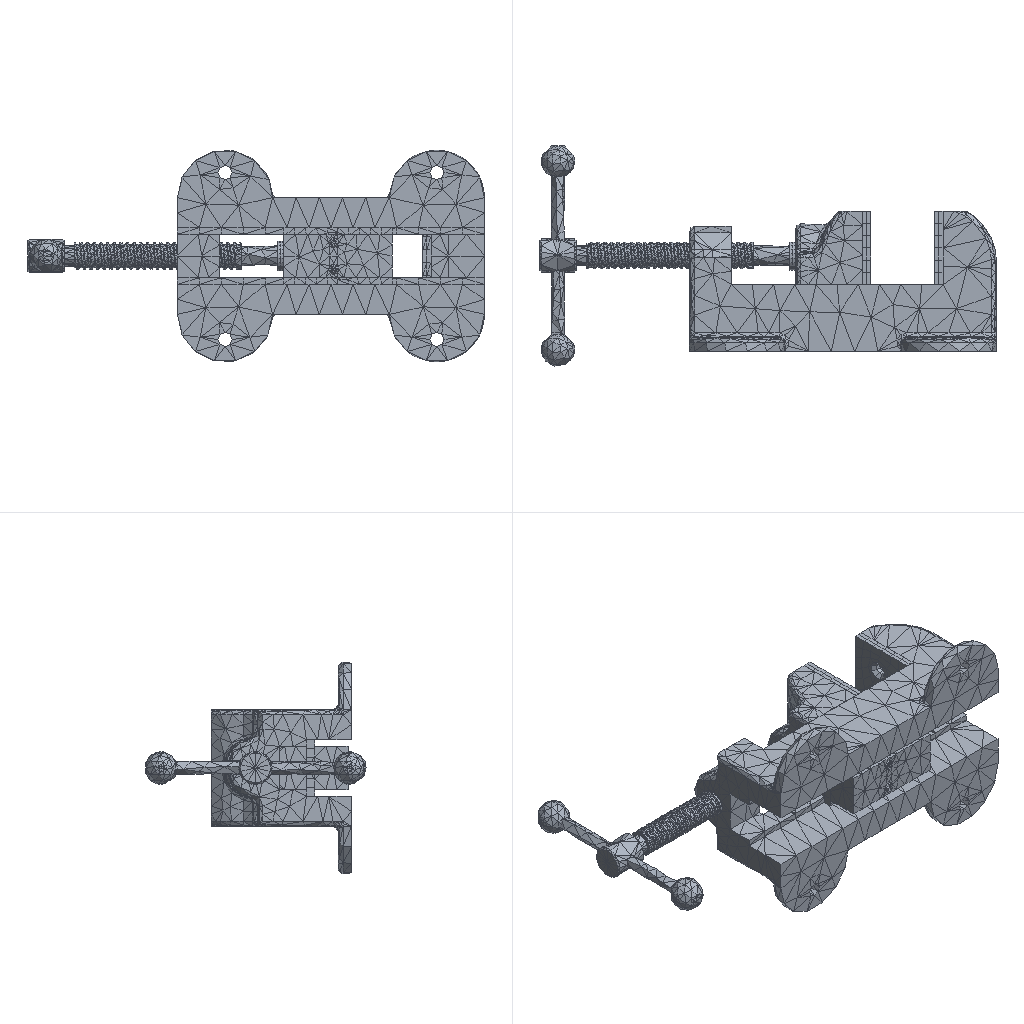Simulation study | ansys workbench
Ansys APDL input file, long lists of numbers shortened:
/batch
/config,noeldb,1     ! force off writing results to database
*get,_wallstrt,active,,time,wall
! ANSYS input file written by Workbench version 2022 R1
! File used for geometry attach:
/title,wbnew--____ (B5)
! ****** Begin Custom Load Command Snippet ******
/COM, ACT Extensions:
/COM,     LSDYNA, 2021.1
/COM,
! ****** End   Custom Load Command Snippet ******
*DIM,_wb_ProjectScratch_dir,string,248
_wb_ProjectScratch_dir(1) = ''
*DIM,_wb_SolverFiles_dir,string,248
_wb_SolverFiles_dir(1) = ''
*DIM,_wb_userfiles_dir,string,248
_wb_userfiles_dir(1) = ''
/com,--- Data in consistent NMM units. See Solving Units in the help system for more information.
/units,MPA
/nopr
/wb,file,start              !  signify a WB generated input file
/prep7
! Turn off shape checking because checks already performed inside WB mesher.
! See help system for more information.
SHPP,OFF,,NOWARN
/nolist
etcon,set             ! allow ANSYS to choose best KEYOP's for 180x elements, resets any applicable keyopt to MAPDL defaults
/com,*********** Nodes for the whole assembly ***********
nblock,3,,58891
(1i9,3e20.9e3)
        1    -1.019636445E+02     8.701916000E+00    -9.855497806E-15
! (53537 more lines like these left out)
-1
/wb,elem,start            !  set before creation of elements
/com,*********** Elements for Body 1 "_model4|_model4" ***********
et,1,187
eblock,19,solid,,3611
(19i9)
        1        1        1        1        0        0        0        0       10        0     7530    18194    18549    18359    18458    22945    23774    22940    22943
! (7221 more lines like these left out)
-1
/com,*********** Elements for Body 2 "_model19|_model19" ***********
et,2,186
keyo,2,2,1          ! set full integration on SOLID186
eblock,19,solid,,130
(19i9)
        2        2        2        2        0        0        0        0       20        0     4919    11682    11703    11701    11704    11757    11736    11738    11735
! (259 more lines like these left out)
-1
/com,*********** Elements for Body 3 "_model3|_model3" ***********
et,3,187
eblock,19,solid,,2042
(19i9)
        3        3        3        3        0        0        0        0       10        0    13595    29093    29183    29390    29313    31163    31664    31165    31164
! (4083 more lines like these left out)
-1
/com,*********** Elements for Body 4 "_model3|_model3[2]" ***********
et,4,187
eblock,19,solid,,3162
(19i9)
        4        4        4        4        0        0        0        0       10        0     1757     6861     7168     7270     7266     9651    11542     9656     9655
! (6323 more lines like these left out)
-1
/com,*********** Elements for Body 5 "_model19|_model19[2]" ***********
et,5,186
keyo,5,2,1          ! set full integration on SOLID186
eblock,19,solid,,130
(19i9)
        5        5        5        5        0        0        0        0       20        0     1123     2851     2872     2870     2873     2926     2905     2907     2904
! (259 more lines like these left out)
-1
! (12 more sections like these left out)
/wb,elem,end               !  done creating elements
/com,*********** Send User Defined Coordinate System(s) ***********
csys,0
toffst,273.15,  ! Temperature offset from absolute zero
/com,*********** Set Reference Temperature ***********
tref,22.
/wb,mat,start              !  starting to send materials
/com,*********** Send Materials ***********
Temperature = 'TEMP' ! Temperature
MP,DENS,1,7.85e-09,	! tonne mm^-3
MP,ALPX,1,1.2e-05,	! C^-1
MP,C,1,434000000,	! mm^2 s^-2 C^-1
MP,KXX,1,60.5,	! tonne mm s^-3 C^-1
MP,RSVX,1,0.00017,	! ohm mm
MP,EX,1,200000,	! tonne s^-2 mm^-1
MP,NUXY,1,0.3,
MP,MURX,1,10000,
Temperature = 'TEMP' ! Temperature
MP,DENS,2,7.85e-09,	! tonne mm^-3
MP,ALPX,2,1.2e-05,	! C^-1
MP,C,2,434000000,	! mm^2 s^-2 C^-1
MP,KXX,2,60.5,	! tonne mm s^-3 C^-1
MP,RSVX,2,0.00017,	! ohm mm
MP,EX,2,200000,	! tonne s^-2 mm^-1
MP,NUXY,2,0.3,
MP,MURX,2,10000,
Temperature = 'TEMP' ! Temperature
MP,DENS,3,7.85e-09,	! tonne mm^-3
MP,ALPX,3,1.2e-05,	! C^-1
MP,C,3,434000000,	! mm^2 s^-2 C^-1
MP,KXX,3,60.5,	! tonne mm s^-3 C^-1
MP,RSVX,3,0.00017,	! ohm mm
MP,EX,3,200000,	! tonne s^-2 mm^-1
MP,NUXY,3,0.3,
MP,MURX,3,10000,
Temperature = 'TEMP' ! Temperature
MP,DENS,4,7.85e-09,	! tonne mm^-3
MP,ALPX,4,1.2e-05,	! C^-1
MP,C,4,434000000,	! mm^2 s^-2 C^-1
MP,KXX,4,60.5,	! tonne mm s^-3 C^-1
MP,RSVX,4,0.00017,	! ohm mm
MP,EX,4,200000,	! tonne s^-2 mm^-1
MP,NUXY,4,0.3,
MP,MURX,4,10000,
Temperature = 'TEMP' ! Temperature
MP,DENS,5,7.85e-09,	! tonne mm^-3
MP,ALPX,5,1.2e-05,	! C^-1
MP,C,5,434000000,	! mm^2 s^-2 C^-1
MP,KXX,5,60.5,	! tonne mm s^-3 C^-1
MP,RSVX,5,0.00017,	! ohm mm
MP,EX,5,200000,	! tonne s^-2 mm^-1
MP,NUXY,5,0.3,
MP,MURX,5,10000,
Temperature = 'TEMP' ! Temperature
MP,DENS,6,7.85e-09,	! tonne mm^-3
MP,ALPX,6,1.2e-05,	! C^-1
MP,C,6,434000000,	! mm^2 s^-2 C^-1
MP,KXX,6,60.5,	! tonne mm s^-3 C^-1
MP,RSVX,6,0.00017,	! ohm mm
MP,EX,6,200000,	! tonne s^-2 mm^-1
MP,NUXY,6,0.3,
MP,MURX,6,10000,
Temperature = 'TEMP' ! Temperature
MP,DENS,7,7.85e-09,	! tonne mm^-3
MP,ALPX,7,1.2e-05,	! C^-1
MP,C,7,434000000,	! mm^2 s^-2 C^-1
MP,KXX,7,60.5,	! tonne mm s^-3 C^-1
MP,RSVX,7,0.00017,	! ohm mm
MP,EX,7,200000,	! tonne s^-2 mm^-1
MP,NUXY,7,0.3,
MP,MURX,7,10000,
Temperature = 'TEMP' ! Temperature
MP,DENS,8,7.85e-09,	! tonne mm^-3
MP,ALPX,8,1.2e-05,	! C^-1
MP,C,8,434000000,	! mm^2 s^-2 C^-1
MP,KXX,8,60.5,	! tonne mm s^-3 C^-1
MP,RSVX,8,0.00017,	! ohm mm
MP,EX,8,200000,	! tonne s^-2 mm^-1
MP,NUXY,8,0.3,
MP,MURX,8,10000,
Temperature = 'TEMP' ! Temperature
MP,DENS,9,7.85e-09,	! tonne mm^-3
MP,ALPX,9,1.2e-05,	! C^-1
MP,C,9,434000000,	! mm^2 s^-2 C^-1
MP,KXX,9,60.5,	! tonne mm s^-3 C^-1
MP,RSVX,9,0.00017,	! ohm mm
MP,EX,9,200000,	! tonne s^-2 mm^-1
! (74 more lines like these left out)
/wb,mat,end                !  done sending materials
!************************* Model Summary ********************
!_model4|_model4,	Q235,	matid,	1
!_model19|_model19,	Q235,	matid,	2
!_model3|_model3,	Q235,	matid,	3
!_model3|_model3[2],	Q235,	matid,	4
!_model19|_model19[2],	Q235,	matid,	5
!_model12|_model12,	Q235,	matid,	6
!_model12|_model12[2],	Q235,	matid,	7
!_model20|_model20,	Q235,	matid,	8
!_model25|_model25,	Q235,	matid,	9
!_model27|_model27,	Q235,	matid,	10
!_model27|_model27[2],	Q235,	matid,	11
!_model29|_model29,	Q235,	matid,	12
!_model29|_model29[2],	Q235,	matid,	13
!_model21|_model21,	Q235,	matid,	14
!_model18|_model18,	Q235,	matid,	15
!_model18|_model18[2],	Q235,	matid,	16
!_model127|_model127,	Q235,	matid,	17
!************************* End Model Summary ********************
! get the diagonal of the bounding box. Needed later for other things
*get,_xmin,node,,mnloc,x
*get,_ymin,node,,mnloc,y
*get,_zmin,node,,mnloc,z
*get,_xmax,node,,mxloc,x
*get,_ymax,node,,mxloc,y
*get,_zmax,node,,mxloc,z
_ASMDIAG=(_xmax-_xmin)*(_xmax-_xmin)+(_ymax-_ymin)*(_ymax-_ymin)+(_zmax-_zmin)*(_zmax-_zmin)
_ASMDIAG=SQRT(_ASMDIAG)
/wb,contact,start          !  starting to send contact
/com,*********** Create Contact "接触区域" ***********
/com,            Real Constant Set For Above Contact Is 19 & 18
*set,tid,19
*set,cid,18
r,tid
r,cid
et,tid,170
et,cid,174
eblock,10,,,122
(15i9)
    40517       19       19       19        0    17573    17635    17636    17636    19670    20058    17636    19671
! (121 more lines like these left out)
-1
eblock,10,,,122
(15i9)
    40639       18       18       18        0    17573    17635    17636    17636    19670    20058    17636    19671
! (121 more lines like these left out)
-1
eblock,10,,,81
(15i9)
    40761       18       19       18        0    11840    11862    11860    11841    12424    12459    12426    12423
! (80 more lines like these left out)
-1
eblock,10,,,81
(15i9)
    40842       19       18       19        0    11840    11862    11860    11841    12424    12459    12426    12423
! (80 more lines like these left out)
-1
keyo,cid,8,2               ! auto create asymmetric contact (from Program Controlled setting)
keyo,cid,10,0              ! adjust contact stiffness each NR iteration (from Program Controlled setting)
keyo,cid,12,5              ! bonded always
keyo,cid,18,1              ! small sliding turned on by application
keyo,cid,2,0               ! augmented Lagrange (from Program Controlled setting)
keyo,cid,4,0               ! on Gauss point (from Program Controlled setting)
keyo,cid,9,1               ! ignore initial gaps/penetration
keyo,cid,7,0               ! No Prediction
rmod,tid,3,10.      ! FKN
rmod,tid,5,0.       ! ICONT
rmod,tid,6,0.       ! PINB
rmod,tid,10,0.      ! CNOF
rmod,tid,12,0.      ! FKT
rmod,tid,36,74      ! WB DSID
rmod,cid,3,10.      ! FKN
rmod,cid,5,0.       ! ICONT
rmod,cid,6,0.       ! PINB
rmod,cid,10,0.      ! CNOF
rmod,cid,12,0.      ! FKT
rmod,cid,36,74      ! WB DSID
/com,*********** Create Contact "接触区域 2" ***********
/com,            Real Constant Set For Above Contact Is 21 & 20
*set,tid,21
*set,cid,20
r,tid
r,cid
et,tid,170
et,cid,174
eblock,10,,,44
(15i9)
    40923       21       21       21        0    17642    17578    17641    17641    19705    19704    17641    20098
! (43 more lines like these left out)
-1
eblock,10,,,44
(15i9)
    40967       20       20       20        0    17642    17578    17641    17641    19705    19704    17641    20098
! (43 more lines like these left out)
-1
eblock,10,,,82
(15i9)
    41011       20       21       20        0    28931    28932    29239    29239    30220    30228    29239    30224
! (81 more lines like these left out)
-1
eblock,10,,,82
(15i9)
    41093       21       20       21        0    28931    28932    29239    29239    30220    30228    29239    30224
! (81 more lines like these left out)
-1
keyo,cid,8,2               ! auto create asymmetric contact (from Program Controlled setting)
keyo,cid,10,0              ! adjust contact stiffness each NR iteration (from Program Controlled setting)
keyo,cid,12,5              ! bonded always
keyo,cid,18,1              ! small sliding turned on by application
keyo,cid,2,0               ! augmented Lagrange (from Program Controlled setting)
keyo,cid,4,0               ! on Gauss point (from Program Controlled setting)
keyo,cid,9,1               ! ignore initial gaps/penetration
keyo,cid,7,0               ! No Prediction
rmod,tid,3,10.      ! FKN
rmod,tid,5,0.       ! ICONT
rmod,tid,6,0.       ! PINB
rmod,tid,10,0.      ! CNOF
rmod,tid,12,0.      ! FKT
rmod,tid,36,77      ! WB DSID
rmod,cid,3,10.      ! FKN
rmod,cid,5,0.       ! ICONT
rmod,cid,6,0.       ! PINB
rmod,cid,10,0.      ! CNOF
rmod,cid,12,0.      ! FKT
rmod,cid,36,77      ! WB DSID
/com,*********** Create Contact "接触区域 3" ***********
/com,            Real Constant Set For Above Contact Is 23 & 22
*set,tid,23
*set,cid,22
r,tid
r,cid
et,tid,170
et,cid,174
eblock,10,,,4
(15i9)
    41175       23       23       23        0    17576    17575    17639    17639    19683    19685    17639    19691
    41176       23       23       23        0    17639    17575    17638    17638    19685    19684    17638    20083
    41177       23       23       23        0    17765    17435    17436    17436    18724    18723    17436    18732
    41178       23       23       23        0    17766    17435    17765    17765    18725    18724    17765    20878
-1
eblock,10,,,4
(15i9)
    41179       22       22       22        0    17576    17575    17639    17639    19683    19685    17639    19691
    41180       22       22       22        0    17639    17575    17638    17638    19685    19684    17638    20083
    41181       22       22       22        0    17765    17435    17436    17436    18724    18723    17436    18732
    41182       22       22       22        0    17766    17435    17765    17765    18725    18724    17765    20878
-1
eblock,10,,,16
(15i9)
    41183       22       23       22        0     3009     3031     3029     3010     3593     3628     3595     3592
! (15 more lines like these left out)
-1
eblock,10,,,16
(15i9)
    41199       23       22       23        0     3009     3031     3029     3010     3593     3628     3595     3592
! (15 more lines like these left out)
-1
keyo,cid,8,2               ! auto create asymmetric contact (from Program Controlled setting)
keyo,cid,10,0              ! adjust contact stiffness each NR iteration (from Program Controlled setting)
keyo,cid,12,5              ! bonded always
keyo,cid,18,1              ! small sliding turned on by application
keyo,cid,2,0               ! augmented Lagrange (from Program Controlled setting)
keyo,cid,4,0               ! on Gauss point (from Program Controlled setting)
keyo,cid,9,1               ! ignore initial gaps/penetration
keyo,cid,7,0               ! No Prediction
rmod,tid,3,10.      ! FKN
rmod,tid,5,0.       ! ICONT
rmod,tid,6,0.       ! PINB
rmod,tid,10,0.      ! CNOF
rmod,tid,12,0.      ! FKT
rmod,tid,36,80      ! WB DSID
rmod,cid,3,10.      ! FKN
rmod,cid,5,0.       ! ICONT
rmod,cid,6,0.       ! PINB
rmod,cid,10,0.      ! CNOF
rmod,cid,12,0.      ! FKT
rmod,cid,36,80      ! WB DSID
/com,*********** Create Contact "接触区域 4" ***********
/com,            Real Constant Set For Above Contact Is 25 & 24
*set,tid,25
*set,cid,24
r,tid
r,cid
et,tid,170
et,cid,174
eblock,10,,,24
(15i9)
    41215       25       25       25        0    17612    17872    17873    17873    19926    21474    17873    19927
! (23 more lines like these left out)
-1
eblock,10,,,24
(15i9)
    41239       24       24       24        0    17612    17872    17873    17873    19926    21474    17873    19927
! (23 more lines like these left out)
-1
eblock,10,,,35
(15i9)
    41263       24       25       24        0     2613     2614     2661     2662     2771     2774     2844     2772
! (34 more lines like these left out)
-1
eblock,10,,,35
(15i9)
    41298       25       24       25        0     2613     2614     2661     2662     2771     2774     2844     2772
! (34 more lines like these left out)
-1
keyo,cid,8,2               ! auto create asymmetric contact (from Program Controlled setting)
keyo,cid,10,0              ! adjust contact stiffness each NR iteration (from Program Controlled setting)
keyo,cid,12,5              ! bonded always
keyo,cid,18,1              ! small sliding turned on by application
keyo,cid,2,0               ! augmented Lagrange (from Program Controlled setting)
keyo,cid,4,0               ! on Gauss point (from Program Controlled setting)
keyo,cid,9,1               ! ignore initial gaps/penetration
keyo,cid,7,0               ! No Prediction
rmod,tid,3,10.      ! FKN
rmod,tid,5,0.       ! ICONT
rmod,tid,6,0.       ! PINB
rmod,tid,10,0.      ! CNOF
rmod,tid,12,0.      ! FKT
rmod,tid,36,83      ! WB DSID
rmod,cid,3,10.      ! FKN
rmod,cid,5,0.       ! ICONT
rmod,cid,6,0.       ! PINB
rmod,cid,10,0.      ! CNOF
rmod,cid,12,0.      ! FKT
rmod,cid,36,83      ! WB DSID
/com,*********** Create Contact "接触区域 5" ***********
/com,            Real Constant Set For Above Contact Is 27 & 26
*set,tid,27
*set,cid,26
r,tid
r,cid
et,tid,170
et,cid,174
eblock,10,,,24
(15i9)
    41333       27       27       27        0    17911    17897    17910    17910    21584    21583    17910    21642
! (23 more lines like these left out)
-1
eblock,10,,,24
(15i9)
    41357       26       26       26        0    17911    17897    17910    17910    21584    21583    17910    21642
! (23 more lines like these left out)
-1
eblock,10,,,35
(15i9)
    41381       26       27       26        0    12588    12587    12582    12594    12693    12668    12670    12698
! (34 more lines like these left out)
-1
eblock,10,,,35
(15i9)
    41416       27       26       27        0    12588    12587    12582    12594    12693    12668    12670    12698
! (34 more lines like these left out)
-1
keyo,cid,8,2               ! auto create asymmetric contact (from Program Controlled setting)
keyo,cid,10,0              ! adjust contact stiffness each NR iteration (from Program Controlled setting)
keyo,cid,12,5              ! bonded always
keyo,cid,18,1              ! small sliding turned on by application
keyo,cid,2,0               ! augmented Lagrange (from Program Controlled setting)
keyo,cid,4,0               ! on Gauss point (from Program Controlled setting)
keyo,cid,9,1               ! ignore initial gaps/penetration
keyo,cid,7,0               ! No Prediction
rmod,tid,3,10.      ! FKN
rmod,tid,5,0.       ! ICONT
rmod,tid,6,0.       ! PINB
rmod,tid,10,0.      ! CNOF
rmod,tid,12,0.      ! FKT
rmod,tid,36,86      ! WB DSID
rmod,cid,3,10.      ! FKN
rmod,cid,5,0.       ! ICONT
rmod,cid,6,0.       ! PINB
rmod,cid,10,0.      ! CNOF
rmod,cid,12,0.      ! FKT
rmod,cid,36,86      ! WB DSID
! (21 more sections like these left out)
/wb,contact,end            !  done creating contacts
/golist
/wb,load,start             !  starting to send loads
/com,*********** Fixed Supports ***********
CMBLOCK,_FIXEDSU,NODE,      420
(8i10)
     17411     17412     17413     17414     17510     17511     17512     17523
! (52 more lines like these left out)
cmsel,s,_FIXEDSU
d,all,all
nsel,all
/com,*********** Define Force Using Surface Effect Elements ***********
local,12,0,0.,0.,0.,0.,0.,0.
csys,0
et,70,154
eblock,10,,,65
(15i9)
    51685       70       70       70       12     2907     2904     2926     2905     3351     3352     3356     3354
! (64 more lines like these left out)
-1
esel,s,type,,70
keyop,70,2,1                ! Apply load in local coordinate system
keyop,70,7,1                ! Use original area so load is constant in large deformation
esel,all
/com,*********** Define Force Using Surface Effect Elements ***********
local,13,0,0.,0.,0.,0.,0.,0.
csys,0
et,71,154
eblock,10,,,65
(15i9)
    51750       71       71       71       13    11738    11735    11757    11736    12182    12183    12187    12185
! (64 more lines like these left out)
-1
esel,s,type,,71
keyop,71,2,1                ! Apply load in local coordinate system
keyop,71,7,1                ! Use original area so load is constant in large deformation
esel,all
/com,*********** Define Force Using Surface Effect Elements ***********
local,14,0,0.,0.,0.,0.,0.,0.
csys,0
et,72,154
eblock,10,,,52
(15i9)
    51815       72       72       72       14    17767    17434    17766    17766    18718    18717    17766    20883
! (51 more lines like these left out)
-1
esel,s,type,,72
keyop,72,2,1                ! Apply load in local coordinate system
keyop,72,7,1                ! Use original area so load is constant in large deformation
esel,all
/gst,on,on
fini
*get,_numnode,node,0,count
*get,_numelem,elem,0,count
*get, _MAXELEMNUM, elem, 0, NUM, MAX
*get, _MAXNODENUM, node, 0, NUM, MAX
*get, _MAXELEMTYPE, etyp, 0, NUM, MAX
*get, _MAXREALCONST, real, 0, NUM, MAX
/go
/wb,load,end               !  done creating loads
/com,--- Number of total nodes = %_numnode%
/com,--- Number of contact elements = 11350
/com,--- Number of spring elements = 0
/com,--- Number of bearing elements = 0
/com,--- Number of solid elements = 26714
/com,--- Number of condensed parts = 0
/com,--- Number of total elements = %_numelem%
*get,_wallbsol,active,,time,wall
/com,****************************************************************************
/com,*************************    SOLUTION       ********************************
/com,****************************************************************************
/solu
antype,0                   ! static analysis
_thickRatio=0.471   ! Ratio of thick parts in the model
eqsl,sparse,,,,,1
cntr,print,1               ! print out contact info and also make no initial contact an error
dmpoption,emat,no             ! Don't combine emat file for DANSYS
dmpoption,esav,no             ! Don't combine esav file for DANSYS
nldiag,cont,iter           ! print out contact info each equilibrium iteration
rescontrol,,none                 ! Do not keep any restart files
/com,****************************************************
/com,******************* SOLVE FOR LS 1 OF 1 ****************
esel,s,type,,70
nsle
sfe,all,1,pres,1,-1.743
sfe,all,2,pres,1,6.79741685546266e-014
sfe,all,3,pres,1,6.97170980354487e-015
esel,s,type,,71
nsle
sfe,all,1,pres,1,1.743
sfe,all,2,pres,1,0.
sfe,all,3,pres,1,6.97170980354487e-015
esel,s,type,,72
nsle
sfe,all,1,pres,1,0.
sfe,all,2,pres,1,-0.8948
sfe,all,3,pres,1,0.
nsel,all
esel,all
/nopr
/gopr
nsub,1,1,1
time,1.
outres,erase
outres,all,none
outres,nsol,all,
outres,rsol,all
outres,eangl,all
outres,etmp,all
outres,veng,all
outres,strs,all,
outres,epel,all,
outres,eppl,all,
outres,cont,all,
! *********** WB SOLVE COMMAND ***********
! check interactive state
*get,ANSINTER_,active,,int
*if,ANSINTER_,ne,0,then
/eof
*endif
solve
/com *************** Write FE CONNECTORS *********
CEWRITE,file,ce,,INTE
/com,****************************************************
/com,*************** FINISHED SOLVE FOR LS 1 *************
*get,_wallasol,active,,time,wall
/nopr
*get,_numnode,node,0,count
*get,_numelem,elem,0,count
*get, _MAXELEMNUM, elem, 0, NUM, MAX
*get, _MAXNODENUM, node, 0, NUM, MAX,,,INTERNAL
*get, _MAXELEMTYPE, etyp, 0, NUM, MAX
*get, _MAXREALCONST, real, 0, NUM, MAX
/gopr
/post1
xmlo,ENCODING,ISO-8859-1
xmlo,parm
/xml,parm,xml
fini
/gopr
*get,_walldone,active,,time,wall
_preptime=(_wallbsol-_wallstrt)*3600
_solvtime=(_wallasol-_wallbsol)*3600
_posttime=(_walldone-_wallasol)*3600
_totaltim=(_walldone-_wallstrt)*3600
*get,_dlbratio,active,0,solu,dlbr
*get,_combtime,active,0,solu,comb
*get,_ssmode,active,0,solu,ssmm
*get,_ndofs,active,0,solu,ndof
*get,_sol_end_time,active,0,set,time
*if,_sol_end_time,eq,1.,then
/fclean				!clean distributed files
*endif
/com,--- Total number of nodes = %_numnode%
/com,--- Total number of elements = %_numelem%
/com,--- Element load balance ratio = %_dlbratio%
/com,--- Time to combine distributed files = %_combtime%
/com,--- Sparse memory mode = %_ssmode%
/com,--- Number of DOF = %_ndofs%
/wb,file,end               ! done with WB generated input